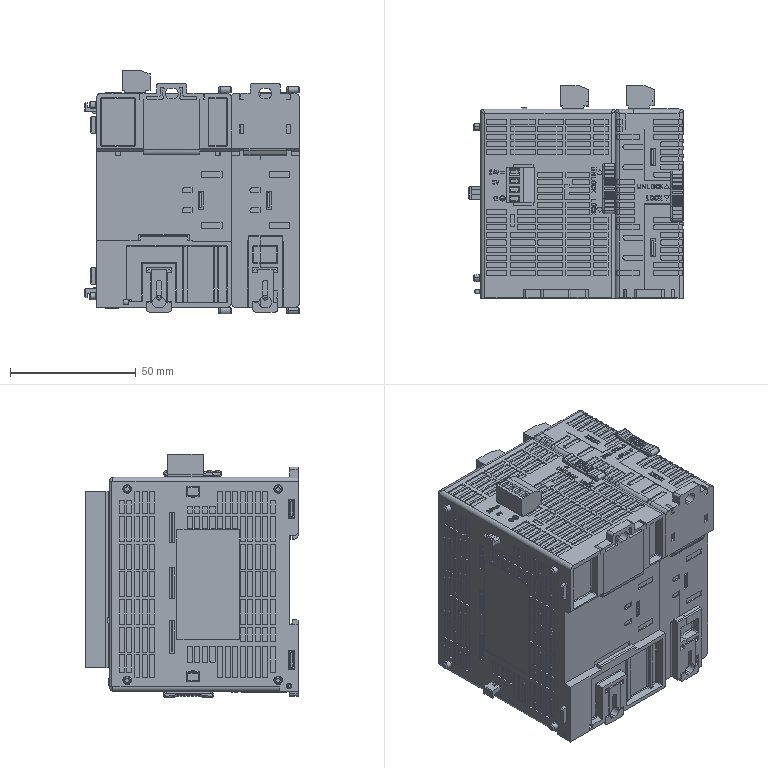Part | SolidWorks | 2 solids | 9732 faces | volume 494108 mm3 | plane 6696 | cylinder 2742 | cone 187 | torus 45 | spline 40 | sphere 22 | commonest cylinder face diameters 0.4 x2017 1 x157 0.6 x113 2.6 x105 2.4 x76 2.8 x74